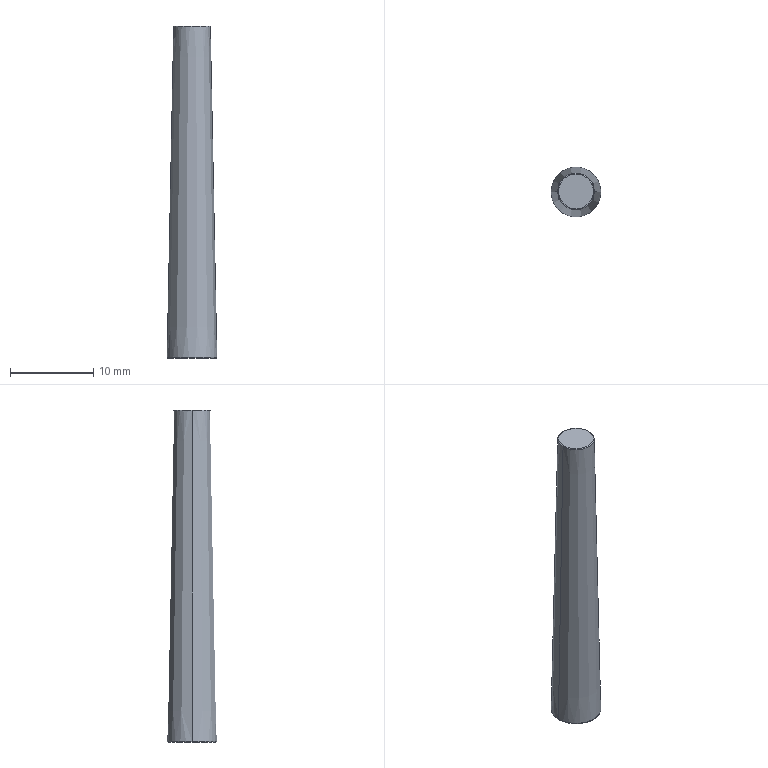Part | SolidWorks | features Extrusion 1, Fillet 1 | 1 solid | 8 faces | box 5.996 x 5.996 x 40 mm | volume 857.367 mm3 | torus 4 | cone 2 | plane 2
STEP:
#1=CARTESIAN_POINT('',(-2.206,0.,39.902));
#2=VERTEX_POINT('',#1);
#3=CARTESIAN_POINT('',(2.206,0.,39.902));
#4=VERTEX_POINT('',#3);
#5=CARTESIAN_POINT('',(0.,0.,39.902));
#6=DIRECTION('',(0.,0.,-1.));
#7=DIRECTION('',(-1.,0.,0.));
#8=AXIS2_PLACEMENT_3D('',#5,#6,#7);
#9=CIRCLE('',#8,2.206);
#10=EDGE_CURVE('',#2,#4,#9,.T.);
#11=ORIENTED_EDGE('',*,*,#10,.F.);
#12=CARTESIAN_POINT('',(-2.106,0.,40.));
#13=VERTEX_POINT('',#12);
#14=CARTESIAN_POINT('',(-2.106,0.,39.9));
#15=DIRECTION('',(0.,1.,0.));
#16=DIRECTION('',(-1.,0.,0.));
#17=AXIS2_PLACEMENT_3D('',#14,#15,#16);
#18=CIRCLE('',#17,0.1);
#19=EDGE_CURVE('',#2,#13,#18,.T.);
#20=ORIENTED_EDGE('',*,*,#19,.T.);
#21=CARTESIAN_POINT('',(2.106,0.,40.));
#22=VERTEX_POINT('',#21);
#23=CARTESIAN_POINT('',(0.,0.,40.));
#24=DIRECTION('',(0.,0.,1.));
#25=DIRECTION('',(1.,0.,0.));
#26=AXIS2_PLACEMENT_3D('',#23,#24,#25);
#27=CIRCLE('',#26,2.106);
#28=EDGE_CURVE('',#22,#13,#27,.T.);
#29=ORIENTED_EDGE('',*,*,#28,.F.);
#30=CARTESIAN_POINT('',(2.106,0.,39.9));
#31=DIRECTION('',(0.,-1.,0.));
#32=DIRECTION('',(0.,0.,-1.));
#33=AXIS2_PLACEMENT_3D('',#30,#31,#32);
#34=CIRCLE('',#33,0.1);
#35=EDGE_CURVE('',#4,#22,#34,.T.);
#36=ORIENTED_EDGE('',*,*,#35,.F.);
#37=EDGE_LOOP('',(#11,#20,#29,#36));
#38=FACE_OUTER_BOUND('',#37,.T.);
#39=CARTESIAN_POINT('',(0.,0.,39.9));
#40=DIRECTION('',(0.,0.,1.));
#41=DIRECTION('',(1.,0.,0.));
#42=AXIS2_PLACEMENT_3D('',#39,#40,#41);
#43=TOROIDAL_SURFACE('',#42,2.106,0.1);
#44=ADVANCED_FACE('',(#38),#43,.T.);
#45=CARTESIAN_POINT('',(-2.898,0.,0.));
#46=VERTEX_POINT('',#45);
#47=CARTESIAN_POINT('',(2.898,0.,0.));
#48=VERTEX_POINT('',#47);
#49=CARTESIAN_POINT('',(0.,0.,0.));
#50=DIRECTION('',(0.,0.,-1.));
#51=DIRECTION('',(1.,0.,0.));
#52=AXIS2_PLACEMENT_3D('',#49,#50,#51);
#53=CIRCLE('',#52,2.898);
#54=EDGE_CURVE('',#46,#48,#53,.T.);
#55=ORIENTED_EDGE('',*,*,#54,.F.);
#56=CARTESIAN_POINT('',(-2.998,0.,0.102));
#57=VERTEX_POINT('',#56);
#58=CARTESIAN_POINT('',(-2.898,0.,0.1));
#59=DIRECTION('',(0.,1.,0.));
#60=DIRECTION('',(-1.,0.,0.));
#61=AXIS2_PLACEMENT_3D('',#58,#59,#60);
#62=CIRCLE('',#61,0.1);
#63=EDGE_CURVE('',#46,#57,#62,.T.);
#64=ORIENTED_EDGE('',*,*,#63,.T.);
#65=CARTESIAN_POINT('',(2.998,0.,0.102));
#66=VERTEX_POINT('',#65);
#67=CARTESIAN_POINT('',(0.,0.,0.102));
#68=DIRECTION('',(0.,0.,1.));
#69=DIRECTION('',(1.,0.,0.));
#70=AXIS2_PLACEMENT_3D('',#67,#68,#69);
#71=CIRCLE('',#70,2.998);
#72=EDGE_CURVE('',#66,#57,#71,.T.);
#73=ORIENTED_EDGE('',*,*,#72,.F.);
#74=CARTESIAN_POINT('',(2.898,0.,0.1));
#75=DIRECTION('',(0.,-1.,0.));
#76=DIRECTION('',(0.,0.,-1.));
#77=AXIS2_PLACEMENT_3D('',#74,#75,#76);
#78=CIRCLE('',#77,0.1);
#79=EDGE_CURVE('',#48,#66,#78,.T.);
#80=ORIENTED_EDGE('',*,*,#79,.F.);
#81=EDGE_LOOP('',(#55,#64,#73,#80));
#82=FACE_OUTER_BOUND('',#81,.T.);
#83=CARTESIAN_POINT('',(0.,0.,0.1));
#84=DIRECTION('',(0.,0.,1.));
#85=DIRECTION('',(1.,0.,0.));
#86=AXIS2_PLACEMENT_3D('',#83,#84,#85);
#87=TOROIDAL_SURFACE('',#86,2.898,0.1);
#88=ADVANCED_FACE('',(#82),#87,.T.);
#89=CARTESIAN_POINT('',(0.,0.,39.902));
#90=DIRECTION('',(0.,0.,-1.));
#91=DIRECTION('',(-1.,0.,0.));
#92=AXIS2_PLACEMENT_3D('',#89,#90,#91);
#93=CIRCLE('',#92,2.206);
#94=EDGE_CURVE('',#4,#2,#93,.T.);
#95=ORIENTED_EDGE('',*,*,#94,.T.);
#96=CARTESIAN_POINT('',(-3.,0.,0.));
#97=DIRECTION('',(-0.0199,0.,-0.9998));
#98=VECTOR('',#97,1000.);
#99=LINE('',#96,#98);
#100=EDGE_CURVE('',#2,#57,#99,.T.);
#101=ORIENTED_EDGE('',*,*,#100,.T.);
#102=CARTESIAN_POINT('',(0.,0.,0.102));
#103=DIRECTION('',(0.,0.,1.));
#104=DIRECTION('',(1.,0.,0.));
#105=AXIS2_PLACEMENT_3D('',#102,#103,#104);
#106=CIRCLE('',#105,2.998);
#107=EDGE_CURVE('',#57,#66,#106,.T.);
#108=ORIENTED_EDGE('',*,*,#107,.T.);
#109=CARTESIAN_POINT('',(3.,0.,0.));
#110=DIRECTION('',(0.0199,0.,-0.9998));
#111=VECTOR('',#110,1000.);
#112=LINE('',#109,#111);
#113=EDGE_CURVE('',#4,#66,#112,.T.);
#114=ORIENTED_EDGE('',*,*,#113,.F.);
#115=EDGE_LOOP('',(#95,#101,#108,#114));
#116=FACE_OUTER_BOUND('',#115,.T.);
#117=CARTESIAN_POINT('',(0.,0.,0.));
#118=DIRECTION('',(0.,0.,-1.));
#119=DIRECTION('',(1.,0.,0.));
#120=AXIS2_PLACEMENT_3D('',#117,#118,#119);
#121=CONICAL_SURFACE('',#120,3.,0.0199);
#122=ADVANCED_FACE('',(#116),#121,.T.);
#123=ORIENTED_EDGE('',*,*,#100,.F.);
#124=ORIENTED_EDGE('',*,*,#10,.T.);
#125=ORIENTED_EDGE('',*,*,#113,.T.);
#126=ORIENTED_EDGE('',*,*,#72,.T.);
#127=EDGE_LOOP('',(#123,#124,#125,#126));
#128=FACE_OUTER_BOUND('',#127,.T.);
#129=CARTESIAN_POINT('',(0.,0.,0.));
#130=DIRECTION('',(0.,0.,-1.));
#131=DIRECTION('',(1.,0.,0.));
#132=AXIS2_PLACEMENT_3D('',#129,#130,#131);
#133=CONICAL_SURFACE('',#132,3.,0.0199);
#134=ADVANCED_FACE('',(#128),#133,.T.);
#135=ORIENTED_EDGE('',*,*,#28,.T.);
#136=CARTESIAN_POINT('',(0.,0.,40.));
#137=DIRECTION('',(0.,0.,1.));
#138=DIRECTION('',(1.,0.,0.));
#139=AXIS2_PLACEMENT_3D('',#136,#137,#138);
#140=CIRCLE('',#139,2.106);
#141=EDGE_CURVE('',#13,#22,#140,.T.);
#142=ORIENTED_EDGE('',*,*,#141,.T.);
#143=EDGE_LOOP('',(#135,#142));
#144=FACE_OUTER_BOUND('',#143,.T.);
#145=CARTESIAN_POINT('',(0.,0.,40.));
#146=DIRECTION('',(0.,0.,1.));
#147=DIRECTION('',(1.,0.,0.));
#148=AXIS2_PLACEMENT_3D('',#145,#146,#147);
#149=PLANE('',#148);
#150=ADVANCED_FACE('',(#144),#149,.T.);
#151=CARTESIAN_POINT('',(0.,0.,0.));
#152=DIRECTION('',(0.,0.,-1.));
#153=DIRECTION('',(1.,0.,0.));
#154=AXIS2_PLACEMENT_3D('',#151,#152,#153);
#155=CIRCLE('',#154,2.898);
#156=EDGE_CURVE('',#48,#46,#155,.T.);
#157=ORIENTED_EDGE('',*,*,#156,.T.);
#158=ORIENTED_EDGE('',*,*,#54,.T.);
#159=EDGE_LOOP('',(#157,#158));
#160=FACE_OUTER_BOUND('',#159,.T.);
#161=CARTESIAN_POINT('',(0.,0.,0.));
#162=DIRECTION('',(0.,0.,1.));
#163=DIRECTION('',(1.,0.,0.));
#164=AXIS2_PLACEMENT_3D('',#161,#162,#163);
#165=PLANE('',#164);
#166=ADVANCED_FACE('',(#160),#165,.F.);
#167=ORIENTED_EDGE('',*,*,#63,.F.);
#168=ORIENTED_EDGE('',*,*,#156,.F.);
#169=ORIENTED_EDGE('',*,*,#79,.T.);
#170=ORIENTED_EDGE('',*,*,#107,.F.);
#171=EDGE_LOOP('',(#167,#168,#169,#170));
#172=FACE_OUTER_BOUND('',#171,.T.);
#173=CARTESIAN_POINT('',(0.,0.,0.1));
#174=DIRECTION('',(0.,0.,1.));
#175=DIRECTION('',(1.,0.,0.));
#176=AXIS2_PLACEMENT_3D('',#173,#174,#175);
#177=TOROIDAL_SURFACE('',#176,2.898,0.1);
#178=ADVANCED_FACE('',(#172),#177,.T.);
#179=ORIENTED_EDGE('',*,*,#19,.F.);
#180=ORIENTED_EDGE('',*,*,#94,.F.);
#181=ORIENTED_EDGE('',*,*,#35,.T.);
#182=ORIENTED_EDGE('',*,*,#141,.F.);
#183=EDGE_LOOP('',(#179,#180,#181,#182));
#184=FACE_OUTER_BOUND('',#183,.T.);
#185=CARTESIAN_POINT('',(0.,0.,39.9));
#186=DIRECTION('',(0.,0.,1.));
#187=DIRECTION('',(1.,0.,0.));
#188=AXIS2_PLACEMENT_3D('',#185,#186,#187);
#189=TOROIDAL_SURFACE('',#188,2.106,0.1);
#190=ADVANCED_FACE('',(#184),#189,.T.);
#191=CLOSED_SHELL('',(#44,#88,#122,#134,#150,#166,#178,#190));
#192=MANIFOLD_SOLID_BREP('',#191);
#193=CARTESIAN_POINT('',(0.,0.,0.));
#194=DIRECTION('',(0.,0.,1.));
#195=DIRECTION('',(1.,0.,0.));
#196=AXIS2_PLACEMENT_3D('',#193,#194,#195);
#197=(LENGTH_UNIT()NAMED_UNIT(*)SI_UNIT(.MILLI.,.METRE.));
#198=UNCERTAINTY_MEASURE_WITH_UNIT(LENGTH_MEASURE(0.00001),#197,'','');
#199=(NAMED_UNIT(*)PLANE_ANGLE_UNIT()SI_UNIT($,.RADIAN.));
#200=(NAMED_UNIT(*)SI_UNIT($,.STERADIAN.)SOLID_ANGLE_UNIT());
#201=(GEOMETRIC_REPRESENTATION_CONTEXT(3)GLOBAL_UNCERTAINTY_ASSIGNED_CONTEXT((#198))GLOBAL_UNIT_ASSIGNED_CONTEXT((#197,#199,#200))REPRESENTATION_CONTEXT('',''));
#202=ADVANCED_BREP_SHAPE_REPRESENTATION('',(#192,#196),#201);